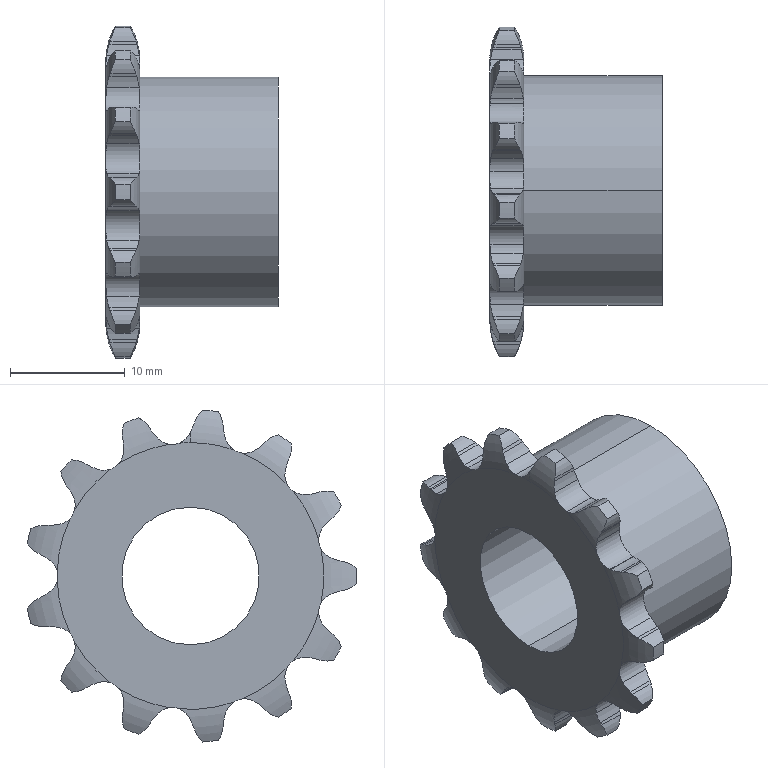Part | SolidWorks | features ICE 3, CirPattern 1, Cut 1, RefAxis 1, Revolution 1 | 1 solid | 147 faces | box 15 x 28.727 x 28.922 mm | volume 3598 mm3 | cylinder 90 | plane 29 | torus 28 | commonest cylinder face diameters 4.824 x29 8.696 x27 3.416 x15 29 x13 3.417 x2 12 x2